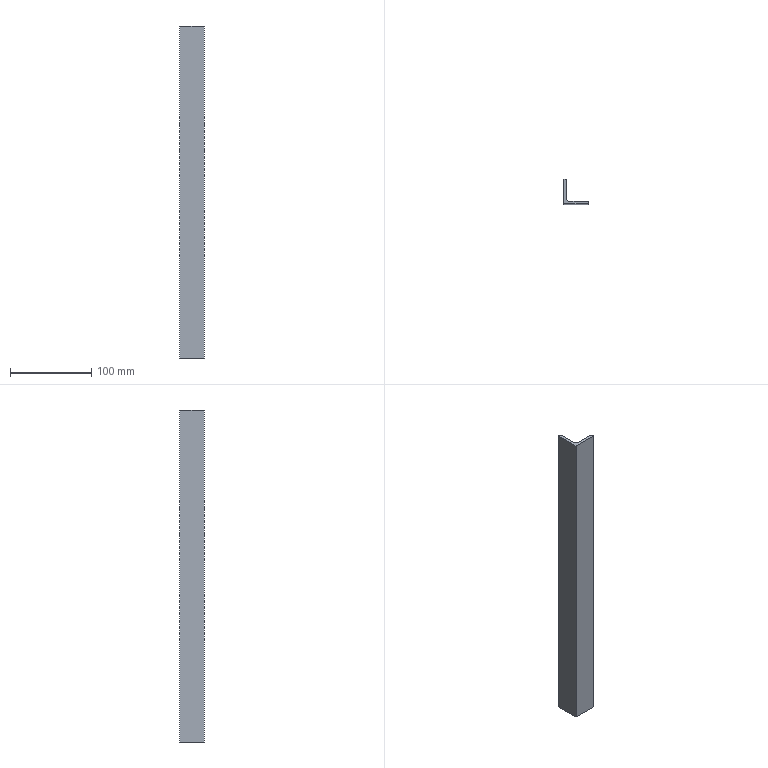Part | SolidWorks | features Extrusion 1 | 1 solid | 11 faces | box 30 x 30 x 407.6 mm | volume 71296 mm3 | plane 8 | cylinder 3 | commonest cylinder face diameters 2 x2 9 x1
STEP:
#1=CARTESIAN_POINT('',(2.,30.,-203.8));
#2=VERTEX_POINT('',#1);
#3=CARTESIAN_POINT('',(3.,29.,-203.8));
#4=VERTEX_POINT('',#3);
#5=CARTESIAN_POINT('',(2.,29.,-203.8));
#6=DIRECTION('',(0.,0.,-1.));
#7=DIRECTION('',(-1.,0.,0.));
#8=AXIS2_PLACEMENT_3D('',#5,#6,#7);
#9=CIRCLE('',#8,1.);
#10=EDGE_CURVE('',#2,#4,#9,.T.);
#11=ORIENTED_EDGE('',*,*,#10,.F.);
#12=CARTESIAN_POINT('',(2.,30.,203.8));
#13=VERTEX_POINT('',#12);
#14=CARTESIAN_POINT('',(2.,30.,203.8));
#15=DIRECTION('',(0.,0.,-1.));
#16=VECTOR('',#15,1000.);
#17=LINE('',#14,#16);
#18=EDGE_CURVE('',#13,#2,#17,.T.);
#19=ORIENTED_EDGE('',*,*,#18,.F.);
#20=CARTESIAN_POINT('',(3.,29.,203.8));
#21=VERTEX_POINT('',#20);
#22=CARTESIAN_POINT('',(2.,29.,203.8));
#23=DIRECTION('',(0.,0.,-1.));
#24=DIRECTION('',(-1.,0.,0.));
#25=AXIS2_PLACEMENT_3D('',#22,#23,#24);
#26=CIRCLE('',#25,1.);
#27=EDGE_CURVE('',#13,#21,#26,.T.);
#28=ORIENTED_EDGE('',*,*,#27,.T.);
#29=CARTESIAN_POINT('',(3.,29.,203.8));
#30=DIRECTION('',(0.,0.,-1.));
#31=VECTOR('',#30,1000.);
#32=LINE('',#29,#31);
#33=EDGE_CURVE('',#21,#4,#32,.T.);
#34=ORIENTED_EDGE('',*,*,#33,.T.);
#35=EDGE_LOOP('',(#11,#19,#28,#34));
#36=FACE_OUTER_BOUND('',#35,.T.);
#37=CARTESIAN_POINT('',(2.,29.,203.8));
#38=DIRECTION('',(0.,0.,-1.));
#39=DIRECTION('',(-1.,0.,0.));
#40=AXIS2_PLACEMENT_3D('',#37,#38,#39);
#41=CYLINDRICAL_SURFACE('',#40,1.);
#42=ADVANCED_FACE('',(#36),#41,.T.);
#43=CARTESIAN_POINT('',(0.,30.,-203.8));
#44=VERTEX_POINT('',#43);
#45=CARTESIAN_POINT('',(0.,30.,-203.8));
#46=DIRECTION('',(1.,0.,0.));
#47=VECTOR('',#46,1000.);
#48=LINE('',#45,#47);
#49=EDGE_CURVE('',#44,#2,#48,.T.);
#50=ORIENTED_EDGE('',*,*,#49,.F.);
#51=CARTESIAN_POINT('',(0.,30.,203.8));
#52=VERTEX_POINT('',#51);
#53=CARTESIAN_POINT('',(0.,30.,203.8));
#54=DIRECTION('',(0.,0.,-1.));
#55=VECTOR('',#54,1000.);
#56=LINE('',#53,#55);
#57=EDGE_CURVE('',#52,#44,#56,.T.);
#58=ORIENTED_EDGE('',*,*,#57,.F.);
#59=CARTESIAN_POINT('',(0.,30.,203.8));
#60=DIRECTION('',(1.,0.,0.));
#61=VECTOR('',#60,1000.);
#62=LINE('',#59,#61);
#63=EDGE_CURVE('',#52,#13,#62,.T.);
#64=ORIENTED_EDGE('',*,*,#63,.T.);
#65=ORIENTED_EDGE('',*,*,#18,.T.);
#66=EDGE_LOOP('',(#50,#58,#64,#65));
#67=FACE_OUTER_BOUND('',#66,.T.);
#68=CARTESIAN_POINT('',(0.,30.,203.8));
#69=DIRECTION('',(0.,1.,0.));
#70=DIRECTION('',(0.,0.,1.));
#71=AXIS2_PLACEMENT_3D('',#68,#69,#70);
#72=PLANE('',#71);
#73=ADVANCED_FACE('',(#67),#72,.T.);
#74=CARTESIAN_POINT('',(0.,0.,-203.8));
#75=VERTEX_POINT('',#74);
#76=CARTESIAN_POINT('',(0.,0.,-203.8));
#77=DIRECTION('',(0.,1.,0.));
#78=VECTOR('',#77,1000.);
#79=LINE('',#76,#78);
#80=EDGE_CURVE('',#75,#44,#79,.T.);
#81=ORIENTED_EDGE('',*,*,#80,.F.);
#82=CARTESIAN_POINT('',(0.,0.,203.8));
#83=VERTEX_POINT('',#82);
#84=CARTESIAN_POINT('',(0.,0.,203.8));
#85=DIRECTION('',(0.,0.,-1.));
#86=VECTOR('',#85,1000.);
#87=LINE('',#84,#86);
#88=EDGE_CURVE('',#83,#75,#87,.T.);
#89=ORIENTED_EDGE('',*,*,#88,.F.);
#90=CARTESIAN_POINT('',(0.,0.,203.8));
#91=DIRECTION('',(0.,1.,0.));
#92=VECTOR('',#91,1000.);
#93=LINE('',#90,#92);
#94=EDGE_CURVE('',#83,#52,#93,.T.);
#95=ORIENTED_EDGE('',*,*,#94,.T.);
#96=ORIENTED_EDGE('',*,*,#57,.T.);
#97=EDGE_LOOP('',(#81,#89,#95,#96));
#98=FACE_OUTER_BOUND('',#97,.T.);
#99=CARTESIAN_POINT('',(0.,0.,203.8));
#100=DIRECTION('',(-1.,0.,0.));
#101=DIRECTION('',(0.,0.,1.));
#102=AXIS2_PLACEMENT_3D('',#99,#100,#101);
#103=PLANE('',#102);
#104=ADVANCED_FACE('',(#98),#103,.T.);
#105=CARTESIAN_POINT('',(30.,0.,-203.8));
#106=VERTEX_POINT('',#105);
#107=CARTESIAN_POINT('',(30.,0.,-203.8));
#108=DIRECTION('',(-1.,0.,0.));
#109=VECTOR('',#108,1000.);
#110=LINE('',#107,#109);
#111=EDGE_CURVE('',#106,#75,#110,.T.);
#112=ORIENTED_EDGE('',*,*,#111,.F.);
#113=CARTESIAN_POINT('',(30.,0.,203.8));
#114=VERTEX_POINT('',#113);
#115=CARTESIAN_POINT('',(30.,0.,203.8));
#116=DIRECTION('',(0.,0.,-1.));
#117=VECTOR('',#116,1000.);
#118=LINE('',#115,#117);
#119=EDGE_CURVE('',#114,#106,#118,.T.);
#120=ORIENTED_EDGE('',*,*,#119,.F.);
#121=CARTESIAN_POINT('',(30.,0.,203.8));
#122=DIRECTION('',(-1.,0.,0.));
#123=VECTOR('',#122,1000.);
#124=LINE('',#121,#123);
#125=EDGE_CURVE('',#114,#83,#124,.T.);
#126=ORIENTED_EDGE('',*,*,#125,.T.);
#127=ORIENTED_EDGE('',*,*,#88,.T.);
#128=EDGE_LOOP('',(#112,#120,#126,#127));
#129=FACE_OUTER_BOUND('',#128,.T.);
#130=CARTESIAN_POINT('',(30.,0.,203.8));
#131=DIRECTION('',(0.,-1.,0.));
#132=DIRECTION('',(0.,0.,-1.));
#133=AXIS2_PLACEMENT_3D('',#130,#131,#132);
#134=PLANE('',#133);
#135=ADVANCED_FACE('',(#129),#134,.T.);
#136=CARTESIAN_POINT('',(30.,2.,-203.8));
#137=VERTEX_POINT('',#136);
#138=CARTESIAN_POINT('',(30.,0.,-203.8));
#139=DIRECTION('',(0.,1.,0.));
#140=VECTOR('',#139,1000.);
#141=LINE('',#138,#140);
#142=EDGE_CURVE('',#106,#137,#141,.T.);
#143=ORIENTED_EDGE('',*,*,#142,.T.);
#144=CARTESIAN_POINT('',(30.,2.,203.8));
#145=VERTEX_POINT('',#144);
#146=CARTESIAN_POINT('',(30.,2.,203.8));
#147=DIRECTION('',(0.,0.,-1.));
#148=VECTOR('',#147,1000.);
#149=LINE('',#146,#148);
#150=EDGE_CURVE('',#145,#137,#149,.T.);
#151=ORIENTED_EDGE('',*,*,#150,.F.);
#152=CARTESIAN_POINT('',(30.,0.,203.8));
#153=DIRECTION('',(0.,1.,0.));
#154=VECTOR('',#153,1000.);
#155=LINE('',#152,#154);
#156=EDGE_CURVE('',#114,#145,#155,.T.);
#157=ORIENTED_EDGE('',*,*,#156,.F.);
#158=ORIENTED_EDGE('',*,*,#119,.T.);
#159=EDGE_LOOP('',(#143,#151,#157,#158));
#160=FACE_OUTER_BOUND('',#159,.T.);
#161=CARTESIAN_POINT('',(30.,0.,203.8));
#162=DIRECTION('',(-1.,0.,0.));
#163=DIRECTION('',(0.,0.,1.));
#164=AXIS2_PLACEMENT_3D('',#161,#162,#163);
#165=PLANE('',#164);
#166=ADVANCED_FACE('',(#160),#165,.F.);
#167=CARTESIAN_POINT('',(29.,3.,-203.8));
#168=VERTEX_POINT('',#167);
#169=CARTESIAN_POINT('',(29.,2.,-203.8));
#170=DIRECTION('',(0.,0.,1.));
#171=DIRECTION('',(1.,0.,0.));
#172=AXIS2_PLACEMENT_3D('',#169,#170,#171);
#173=CIRCLE('',#172,1.);
#174=EDGE_CURVE('',#137,#168,#173,.T.);
#175=ORIENTED_EDGE('',*,*,#174,.T.);
#176=CARTESIAN_POINT('',(29.,3.,203.8));
#177=VERTEX_POINT('',#176);
#178=CARTESIAN_POINT('',(29.,3.,203.8));
#179=DIRECTION('',(0.,0.,-1.));
#180=VECTOR('',#179,1000.);
#181=LINE('',#178,#180);
#182=EDGE_CURVE('',#177,#168,#181,.T.);
#183=ORIENTED_EDGE('',*,*,#182,.F.);
#184=CARTESIAN_POINT('',(29.,2.,203.8));
#185=DIRECTION('',(0.,0.,1.));
#186=DIRECTION('',(1.,0.,0.));
#187=AXIS2_PLACEMENT_3D('',#184,#185,#186);
#188=CIRCLE('',#187,1.);
#189=EDGE_CURVE('',#145,#177,#188,.T.);
#190=ORIENTED_EDGE('',*,*,#189,.F.);
#191=ORIENTED_EDGE('',*,*,#150,.T.);
#192=EDGE_LOOP('',(#175,#183,#190,#191));
#193=FACE_OUTER_BOUND('',#192,.T.);
#194=CARTESIAN_POINT('',(29.,2.,203.8));
#195=DIRECTION('',(0.,0.,-1.));
#196=DIRECTION('',(-1.,0.,0.));
#197=AXIS2_PLACEMENT_3D('',#194,#195,#196);
#198=CYLINDRICAL_SURFACE('',#197,1.);
#199=ADVANCED_FACE('',(#193),#198,.T.);
#200=CARTESIAN_POINT('',(7.5,3.,-203.8));
#201=VERTEX_POINT('',#200);
#202=CARTESIAN_POINT('',(7.5,3.,-203.8));
#203=DIRECTION('',(1.,0.,0.));
#204=VECTOR('',#203,1000.);
#205=LINE('',#202,#204);
#206=EDGE_CURVE('',#201,#168,#205,.T.);
#207=ORIENTED_EDGE('',*,*,#206,.F.);
#208=CARTESIAN_POINT('',(7.5,3.,203.8));
#209=VERTEX_POINT('',#208);
#210=CARTESIAN_POINT('',(7.5,3.,203.8));
#211=DIRECTION('',(0.,0.,-1.));
#212=VECTOR('',#211,1000.);
#213=LINE('',#210,#212);
#214=EDGE_CURVE('',#209,#201,#213,.T.);
#215=ORIENTED_EDGE('',*,*,#214,.F.);
#216=CARTESIAN_POINT('',(7.5,3.,203.8));
#217=DIRECTION('',(1.,0.,0.));
#218=VECTOR('',#217,1000.);
#219=LINE('',#216,#218);
#220=EDGE_CURVE('',#209,#177,#219,.T.);
#221=ORIENTED_EDGE('',*,*,#220,.T.);
#222=ORIENTED_EDGE('',*,*,#182,.T.);
#223=EDGE_LOOP('',(#207,#215,#221,#222));
#224=FACE_OUTER_BOUND('',#223,.T.);
#225=CARTESIAN_POINT('',(7.5,3.,203.8));
#226=DIRECTION('',(0.,1.,0.));
#227=DIRECTION('',(-1.,0.,0.));
#228=AXIS2_PLACEMENT_3D('',#225,#226,#227);
#229=PLANE('',#228);
#230=ADVANCED_FACE('',(#224),#229,.T.);
#231=CARTESIAN_POINT('',(3.,7.5,-203.8));
#232=VERTEX_POINT('',#231);
#233=CARTESIAN_POINT('',(7.5,7.5,-203.8));
#234=DIRECTION('',(0.,0.,-1.));
#235=DIRECTION('',(-1.,0.,0.));
#236=AXIS2_PLACEMENT_3D('',#233,#234,#235);
#237=CIRCLE('',#236,4.5);
#238=EDGE_CURVE('',#201,#232,#237,.T.);
#239=ORIENTED_EDGE('',*,*,#238,.T.);
#240=CARTESIAN_POINT('',(3.,7.5,203.8));
#241=VERTEX_POINT('',#240);
#242=CARTESIAN_POINT('',(3.,7.5,203.8));
#243=DIRECTION('',(0.,0.,-1.));
#244=VECTOR('',#243,1000.);
#245=LINE('',#242,#244);
#246=EDGE_CURVE('',#241,#232,#245,.T.);
#247=ORIENTED_EDGE('',*,*,#246,.F.);
#248=CARTESIAN_POINT('',(7.5,7.5,203.8));
#249=DIRECTION('',(0.,0.,-1.));
#250=DIRECTION('',(-1.,0.,0.));
#251=AXIS2_PLACEMENT_3D('',#248,#249,#250);
#252=CIRCLE('',#251,4.5);
#253=EDGE_CURVE('',#209,#241,#252,.T.);
#254=ORIENTED_EDGE('',*,*,#253,.F.);
#255=ORIENTED_EDGE('',*,*,#214,.T.);
#256=EDGE_LOOP('',(#239,#247,#254,#255));
#257=FACE_OUTER_BOUND('',#256,.T.);
#258=CARTESIAN_POINT('',(7.5,7.5,203.8));
#259=DIRECTION('',(0.,0.,-1.));
#260=DIRECTION('',(-1.,0.,0.));
#261=AXIS2_PLACEMENT_3D('',#258,#259,#260);
#262=CYLINDRICAL_SURFACE('',#261,4.5);
#263=ADVANCED_FACE('',(#257),#262,.F.);
#264=CARTESIAN_POINT('',(3.,29.,-203.8));
#265=DIRECTION('',(0.,-1.,0.));
#266=VECTOR('',#265,1000.);
#267=LINE('',#264,#266);
#268=EDGE_CURVE('',#4,#232,#267,.T.);
#269=ORIENTED_EDGE('',*,*,#268,.F.);
#270=ORIENTED_EDGE('',*,*,#33,.F.);
#271=CARTESIAN_POINT('',(3.,29.,203.8));
#272=DIRECTION('',(0.,-1.,0.));
#273=VECTOR('',#272,1000.);
#274=LINE('',#271,#273);
#275=EDGE_CURVE('',#21,#241,#274,.T.);
#276=ORIENTED_EDGE('',*,*,#275,.T.);
#277=ORIENTED_EDGE('',*,*,#246,.T.);
#278=EDGE_LOOP('',(#269,#270,#276,#277));
#279=FACE_OUTER_BOUND('',#278,.T.);
#280=CARTESIAN_POINT('',(3.,29.,203.8));
#281=DIRECTION('',(1.,0.,0.));
#282=DIRECTION('',(0.,1.,0.));
#283=AXIS2_PLACEMENT_3D('',#280,#281,#282);
#284=PLANE('',#283);
#285=ADVANCED_FACE('',(#279),#284,.T.);
#286=ORIENTED_EDGE('',*,*,#27,.F.);
#287=ORIENTED_EDGE('',*,*,#63,.F.);
#288=ORIENTED_EDGE('',*,*,#94,.F.);
#289=ORIENTED_EDGE('',*,*,#125,.F.);
#290=ORIENTED_EDGE('',*,*,#156,.T.);
#291=ORIENTED_EDGE('',*,*,#189,.T.);
#292=ORIENTED_EDGE('',*,*,#220,.F.);
#293=ORIENTED_EDGE('',*,*,#253,.T.);
#294=ORIENTED_EDGE('',*,*,#275,.F.);
#295=EDGE_LOOP('',(#286,#287,#288,#289,#290,#291,#292,#293,#294));
#296=FACE_OUTER_BOUND('',#295,.T.);
#297=CARTESIAN_POINT('',(2.,29.,203.8));
#298=DIRECTION('',(0.,0.,-1.));
#299=DIRECTION('',(-1.,0.,0.));
#300=AXIS2_PLACEMENT_3D('',#297,#298,#299);
#301=PLANE('',#300);
#302=ADVANCED_FACE('',(#296),#301,.F.);
#303=ORIENTED_EDGE('',*,*,#10,.T.);
#304=ORIENTED_EDGE('',*,*,#268,.T.);
#305=ORIENTED_EDGE('',*,*,#238,.F.);
#306=ORIENTED_EDGE('',*,*,#206,.T.);
#307=ORIENTED_EDGE('',*,*,#174,.F.);
#308=ORIENTED_EDGE('',*,*,#142,.F.);
#309=ORIENTED_EDGE('',*,*,#111,.T.);
#310=ORIENTED_EDGE('',*,*,#80,.T.);
#311=ORIENTED_EDGE('',*,*,#49,.T.);
#312=EDGE_LOOP('',(#303,#304,#305,#306,#307,#308,#309,#310,#311));
#313=FACE_OUTER_BOUND('',#312,.T.);
#314=CARTESIAN_POINT('',(2.,29.,-203.8));
#315=DIRECTION('',(0.,0.,-1.));
#316=DIRECTION('',(-1.,0.,0.));
#317=AXIS2_PLACEMENT_3D('',#314,#315,#316);
#318=PLANE('',#317);
#319=ADVANCED_FACE('',(#313),#318,.T.);
#320=CLOSED_SHELL('',(#42,#73,#104,#135,#166,#199,#230,#263,#285,#302,#319));
#321=MANIFOLD_SOLID_BREP('',#320);
#322=CARTESIAN_POINT('',(0.,0.,0.));
#323=DIRECTION('',(0.,0.,1.));
#324=DIRECTION('',(1.,0.,0.));
#325=AXIS2_PLACEMENT_3D('',#322,#323,#324);
#326=(LENGTH_UNIT()NAMED_UNIT(*)SI_UNIT(.MILLI.,.METRE.));
#327=UNCERTAINTY_MEASURE_WITH_UNIT(LENGTH_MEASURE(0.00001),#326,'','');
#328=(NAMED_UNIT(*)PLANE_ANGLE_UNIT()SI_UNIT($,.RADIAN.));
#329=(NAMED_UNIT(*)SI_UNIT($,.STERADIAN.)SOLID_ANGLE_UNIT());
#330=(GEOMETRIC_REPRESENTATION_CONTEXT(3)GLOBAL_UNCERTAINTY_ASSIGNED_CONTEXT((#327))GLOBAL_UNIT_ASSIGNED_CONTEXT((#326,#328,#329))REPRESENTATION_CONTEXT('',''));
#331=ADVANCED_BREP_SHAPE_REPRESENTATION('',(#321,#325),#330);